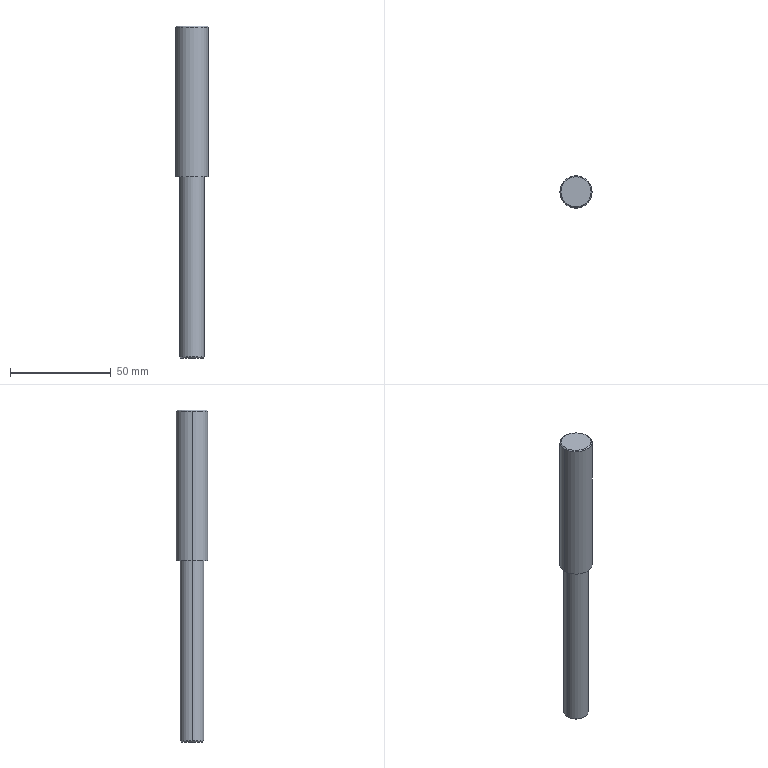Part | STEP file | X77b-01008 | 1 solid | 18 faces | box 16 x 16 x 165 mm | volume 25170 mm3 | cylinder 8 | cone 6 | plane 4 | commonest cylinder face diameters 2.5 x2 3 x2 12 x2 16 x2
STEP:
#1=CARTESIAN_POINT('',(22.255,-49.502,-165.));
#2=VERTEX_POINT('',#1);
#3=CARTESIAN_POINT('',(33.255,-49.502,-165.));
#4=VERTEX_POINT('',#3);
#5=CARTESIAN_POINT('',(27.755,-49.502,-165.));
#6=DIRECTION('',(0.,0.,-1.));
#7=DIRECTION('',(-1.,0.,0.));
#8=AXIS2_PLACEMENT_3D('',#5,#6,#7);
#9=CIRCLE('',#8,5.5);
#10=EDGE_CURVE('',#2,#4,#9,.T.);
#11=ORIENTED_EDGE('',*,*,#10,.F.);
#12=CARTESIAN_POINT('',(21.755,-49.502,-164.5));
#13=VERTEX_POINT('',#12);
#14=CARTESIAN_POINT('',(22.255,-49.502,-165.));
#15=DIRECTION('',(-0.7071,0.,0.7071));
#16=VECTOR('',#15,1000.);
#17=LINE('',#14,#16);
#18=EDGE_CURVE('',#2,#13,#17,.T.);
#19=ORIENTED_EDGE('',*,*,#18,.T.);
#20=CARTESIAN_POINT('',(33.755,-49.502,-164.5));
#21=VERTEX_POINT('',#20);
#22=CARTESIAN_POINT('',(27.755,-49.502,-164.5));
#23=DIRECTION('',(0.,0.,1.));
#24=DIRECTION('',(-1.,0.,0.));
#25=AXIS2_PLACEMENT_3D('',#22,#23,#24);
#26=CIRCLE('',#25,6.);
#27=EDGE_CURVE('',#21,#13,#26,.T.);
#28=ORIENTED_EDGE('',*,*,#27,.F.);
#29=CARTESIAN_POINT('',(33.255,-49.502,-165.));
#30=DIRECTION('',(0.7071,0.,0.7071));
#31=VECTOR('',#30,1000.);
#32=LINE('',#29,#31);
#33=EDGE_CURVE('',#4,#21,#32,.T.);
#34=ORIENTED_EDGE('',*,*,#33,.F.);
#35=EDGE_LOOP('',(#11,#19,#28,#34));
#36=FACE_OUTER_BOUND('',#35,.T.);
#37=CARTESIAN_POINT('',(27.755,-49.502,-165.));
#38=DIRECTION('',(0.,0.,1.));
#39=DIRECTION('',(1.,0.,0.));
#40=AXIS2_PLACEMENT_3D('',#37,#38,#39);
#41=CONICAL_SURFACE('',#40,5.5,0.7854);
#42=ADVANCED_FACE('',(#36),#41,.T.);
#43=CARTESIAN_POINT('',(35.255,-49.502,0.));
#44=VERTEX_POINT('',#43);
#45=CARTESIAN_POINT('',(20.255,-49.502,0.));
#46=VERTEX_POINT('',#45);
#47=CARTESIAN_POINT('',(27.755,-49.502,0.));
#48=DIRECTION('',(0.,0.,1.));
#49=DIRECTION('',(1.,0.,0.));
#50=AXIS2_PLACEMENT_3D('',#47,#48,#49);
#51=CIRCLE('',#50,7.5);
#52=EDGE_CURVE('',#44,#46,#51,.T.);
#53=ORIENTED_EDGE('',*,*,#52,.F.);
#54=CARTESIAN_POINT('',(35.755,-49.502,-0.5));
#55=VERTEX_POINT('',#54);
#56=CARTESIAN_POINT('',(35.255,-49.502,0.));
#57=DIRECTION('',(0.7071,0.,-0.7071));
#58=VECTOR('',#57,1000.);
#59=LINE('',#56,#58);
#60=EDGE_CURVE('',#44,#55,#59,.T.);
#61=ORIENTED_EDGE('',*,*,#60,.T.);
#62=CARTESIAN_POINT('',(19.755,-49.502,-0.5));
#63=VERTEX_POINT('',#62);
#64=CARTESIAN_POINT('',(27.755,-49.502,-0.5));
#65=DIRECTION('',(0.,0.,-1.));
#66=DIRECTION('',(1.,0.,0.));
#67=AXIS2_PLACEMENT_3D('',#64,#65,#66);
#68=CIRCLE('',#67,8.);
#69=EDGE_CURVE('',#63,#55,#68,.T.);
#70=ORIENTED_EDGE('',*,*,#69,.F.);
#71=CARTESIAN_POINT('',(20.255,-49.502,0.));
#72=DIRECTION('',(-0.7071,0.,-0.7071));
#73=VECTOR('',#72,1000.);
#74=LINE('',#71,#73);
#75=EDGE_CURVE('',#46,#63,#74,.T.);
#76=ORIENTED_EDGE('',*,*,#75,.F.);
#77=EDGE_LOOP('',(#53,#61,#70,#76));
#78=FACE_OUTER_BOUND('',#77,.T.);
#79=CARTESIAN_POINT('',(27.755,-49.502,0.));
#80=DIRECTION('',(0.,0.,-1.));
#81=DIRECTION('',(-1.,0.,0.));
#82=AXIS2_PLACEMENT_3D('',#79,#80,#81);
#83=CONICAL_SURFACE('',#82,7.5,0.7854);
#84=ADVANCED_FACE('',(#78),#83,.T.);
#85=CARTESIAN_POINT('',(29.255,-49.502,-157.));
#86=VERTEX_POINT('',#85);
#87=CARTESIAN_POINT('',(26.255,-49.502,-157.));
#88=VERTEX_POINT('',#87);
#89=CARTESIAN_POINT('',(27.755,-49.502,-157.));
#90=DIRECTION('',(0.,0.,-1.));
#91=DIRECTION('',(-1.,0.,0.));
#92=AXIS2_PLACEMENT_3D('',#89,#90,#91);
#93=CIRCLE('',#92,1.5);
#94=EDGE_CURVE('',#86,#88,#93,.T.);
#95=ORIENTED_EDGE('',*,*,#94,.F.);
#96=CARTESIAN_POINT('',(29.255,-49.502,-165.));
#97=VERTEX_POINT('',#96);
#98=CARTESIAN_POINT('',(29.255,-49.502,-165.));
#99=DIRECTION('',(0.,0.,-1.));
#100=VECTOR('',#99,1000.);
#101=LINE('',#98,#100);
#102=EDGE_CURVE('',#86,#97,#101,.T.);
#103=ORIENTED_EDGE('',*,*,#102,.T.);
#104=CARTESIAN_POINT('',(26.255,-49.502,-165.));
#105=VERTEX_POINT('',#104);
#106=CARTESIAN_POINT('',(27.755,-49.502,-165.));
#107=DIRECTION('',(0.,0.,-1.));
#108=DIRECTION('',(-1.,0.,0.));
#109=AXIS2_PLACEMENT_3D('',#106,#107,#108);
#110=CIRCLE('',#109,1.5);
#111=EDGE_CURVE('',#97,#105,#110,.T.);
#112=ORIENTED_EDGE('',*,*,#111,.T.);
#113=CARTESIAN_POINT('',(26.255,-49.502,-165.));
#114=DIRECTION('',(0.,0.,-1.));
#115=VECTOR('',#114,1000.);
#116=LINE('',#113,#115);
#117=EDGE_CURVE('',#88,#105,#116,.T.);
#118=ORIENTED_EDGE('',*,*,#117,.F.);
#119=EDGE_LOOP('',(#95,#103,#112,#118));
#120=FACE_OUTER_BOUND('',#119,.T.);
#121=CARTESIAN_POINT('',(27.755,-49.502,-165.));
#122=DIRECTION('',(0.,0.,-1.));
#123=DIRECTION('',(-1.,0.,0.));
#124=AXIS2_PLACEMENT_3D('',#121,#122,#123);
#125=CYLINDRICAL_SURFACE('',#124,1.5);
#126=ADVANCED_FACE('',(#120),#125,.F.);
#127=CARTESIAN_POINT('',(29.005,-49.502,-153.));
#128=VERTEX_POINT('',#127);
#129=CARTESIAN_POINT('',(26.505,-49.502,-153.));
#130=VERTEX_POINT('',#129);
#131=CARTESIAN_POINT('',(27.755,-49.502,-153.));
#132=DIRECTION('',(0.,0.,-1.));
#133=DIRECTION('',(-1.,0.,0.));
#134=AXIS2_PLACEMENT_3D('',#131,#132,#133);
#135=CIRCLE('',#134,1.25);
#136=EDGE_CURVE('',#128,#130,#135,.T.);
#137=ORIENTED_EDGE('',*,*,#136,.F.);
#138=CARTESIAN_POINT('',(29.005,-49.502,-157.));
#139=VERTEX_POINT('',#138);
#140=CARTESIAN_POINT('',(29.005,-49.502,-165.));
#141=DIRECTION('',(0.,0.,-1.));
#142=VECTOR('',#141,1000.);
#143=LINE('',#140,#142);
#144=EDGE_CURVE('',#128,#139,#143,.T.);
#145=ORIENTED_EDGE('',*,*,#144,.T.);
#146=CARTESIAN_POINT('',(26.505,-49.502,-157.));
#147=VERTEX_POINT('',#146);
#148=CARTESIAN_POINT('',(27.755,-49.502,-157.));
#149=DIRECTION('',(0.,0.,-1.));
#150=DIRECTION('',(-1.,0.,0.));
#151=AXIS2_PLACEMENT_3D('',#148,#149,#150);
#152=CIRCLE('',#151,1.25);
#153=EDGE_CURVE('',#139,#147,#152,.T.);
#154=ORIENTED_EDGE('',*,*,#153,.T.);
#155=CARTESIAN_POINT('',(26.505,-49.502,-165.));
#156=DIRECTION('',(0.,0.,-1.));
#157=VECTOR('',#156,1000.);
#158=LINE('',#155,#157);
#159=EDGE_CURVE('',#130,#147,#158,.T.);
#160=ORIENTED_EDGE('',*,*,#159,.F.);
#161=EDGE_LOOP('',(#137,#145,#154,#160));
#162=FACE_OUTER_BOUND('',#161,.T.);
#163=CARTESIAN_POINT('',(27.755,-49.502,-165.));
#164=DIRECTION('',(0.,0.,-1.));
#165=DIRECTION('',(-1.,0.,0.));
#166=AXIS2_PLACEMENT_3D('',#163,#164,#165);
#167=CYLINDRICAL_SURFACE('',#166,1.25);
#168=ADVANCED_FACE('',(#162),#167,.F.);
#169=CARTESIAN_POINT('',(27.755,-49.502,-152.249));
#170=VERTEX_POINT('',#169);
#171=CARTESIAN_POINT('',(26.505,-49.502,-153.));
#172=DIRECTION('',(-0.8572,0.,-0.515));
#173=VECTOR('',#172,1000.);
#174=LINE('',#171,#173);
#175=EDGE_CURVE('',#170,#130,#174,.T.);
#176=ORIENTED_EDGE('',*,*,#175,.F.);
#177=CARTESIAN_POINT('',(29.005,-49.502,-153.));
#178=DIRECTION('',(0.8572,0.,-0.515));
#179=VECTOR('',#178,1000.);
#180=LINE('',#177,#179);
#181=EDGE_CURVE('',#170,#128,#180,.T.);
#182=ORIENTED_EDGE('',*,*,#181,.T.);
#183=ORIENTED_EDGE('',*,*,#136,.T.);
#184=EDGE_LOOP('',(#176,#182,#183));
#185=FACE_OUTER_BOUND('',#184,.T.);
#186=CARTESIAN_POINT('',(27.755,-49.502,-153.));
#187=DIRECTION('',(0.,0.,-1.));
#188=DIRECTION('',(-1.,0.,0.));
#189=AXIS2_PLACEMENT_3D('',#186,#187,#188);
#190=CONICAL_SURFACE('',#189,1.25,1.03);
#191=ADVANCED_FACE('',(#185),#190,.F.);
#192=ORIENTED_EDGE('',*,*,#27,.T.);
#193=CARTESIAN_POINT('',(21.755,-49.502,-75.));
#194=VERTEX_POINT('',#193);
#195=CARTESIAN_POINT('',(21.755,-49.502,-165.));
#196=DIRECTION('',(0.,0.,1.));
#197=VECTOR('',#196,1000.);
#198=LINE('',#195,#197);
#199=EDGE_CURVE('',#13,#194,#198,.T.);
#200=ORIENTED_EDGE('',*,*,#199,.T.);
#201=CARTESIAN_POINT('',(33.755,-49.502,-75.));
#202=VERTEX_POINT('',#201);
#203=CARTESIAN_POINT('',(27.755,-49.502,-75.));
#204=DIRECTION('',(0.,0.,-1.));
#205=DIRECTION('',(1.,0.,0.));
#206=AXIS2_PLACEMENT_3D('',#203,#204,#205);
#207=CIRCLE('',#206,6.);
#208=EDGE_CURVE('',#194,#202,#207,.T.);
#209=ORIENTED_EDGE('',*,*,#208,.T.);
#210=CARTESIAN_POINT('',(33.755,-49.502,-165.));
#211=DIRECTION('',(0.,0.,1.));
#212=VECTOR('',#211,1000.);
#213=LINE('',#210,#212);
#214=EDGE_CURVE('',#21,#202,#213,.T.);
#215=ORIENTED_EDGE('',*,*,#214,.F.);
#216=EDGE_LOOP('',(#192,#200,#209,#215));
#217=FACE_OUTER_BOUND('',#216,.T.);
#218=CARTESIAN_POINT('',(27.755,-49.502,-165.));
#219=DIRECTION('',(0.,0.,1.));
#220=DIRECTION('',(1.,0.,0.));
#221=AXIS2_PLACEMENT_3D('',#218,#219,#220);
#222=CYLINDRICAL_SURFACE('',#221,6.);
#223=ADVANCED_FACE('',(#217),#222,.T.);
#224=CARTESIAN_POINT('',(35.755,-49.502,-75.));
#225=VERTEX_POINT('',#224);
#226=CARTESIAN_POINT('',(19.755,-49.502,-75.));
#227=VERTEX_POINT('',#226);
#228=CARTESIAN_POINT('',(27.755,-49.502,-75.));
#229=DIRECTION('',(0.,0.,1.));
#230=DIRECTION('',(1.,0.,0.));
#231=AXIS2_PLACEMENT_3D('',#228,#229,#230);
#232=CIRCLE('',#231,8.);
#233=EDGE_CURVE('',#225,#227,#232,.T.);
#234=ORIENTED_EDGE('',*,*,#233,.T.);
#235=CARTESIAN_POINT('',(19.755,-49.502,-75.));
#236=DIRECTION('',(0.,0.,1.));
#237=VECTOR('',#236,1000.);
#238=LINE('',#235,#237);
#239=EDGE_CURVE('',#227,#63,#238,.T.);
#240=ORIENTED_EDGE('',*,*,#239,.T.);
#241=ORIENTED_EDGE('',*,*,#69,.T.);
#242=CARTESIAN_POINT('',(35.755,-49.502,-75.));
#243=DIRECTION('',(0.,0.,1.));
#244=VECTOR('',#243,1000.);
#245=LINE('',#242,#244);
#246=EDGE_CURVE('',#225,#55,#245,.T.);
#247=ORIENTED_EDGE('',*,*,#246,.F.);
#248=EDGE_LOOP('',(#234,#240,#241,#247));
#249=FACE_OUTER_BOUND('',#248,.T.);
#250=CARTESIAN_POINT('',(27.755,-49.502,-75.));
#251=DIRECTION('',(0.,0.,1.));
#252=DIRECTION('',(1.,0.,0.));
#253=AXIS2_PLACEMENT_3D('',#250,#251,#252);
#254=CYLINDRICAL_SURFACE('',#253,8.);
#255=ADVANCED_FACE('',(#249),#254,.T.);
#256=ORIENTED_EDGE('',*,*,#233,.F.);
#257=CARTESIAN_POINT('',(27.755,-49.502,-75.));
#258=DIRECTION('',(0.,0.,1.));
#259=DIRECTION('',(1.,0.,0.));
#260=AXIS2_PLACEMENT_3D('',#257,#258,#259);
#261=CIRCLE('',#260,8.);
#262=EDGE_CURVE('',#227,#225,#261,.T.);
#263=ORIENTED_EDGE('',*,*,#262,.F.);
#264=EDGE_LOOP('',(#256,#263));
#265=FACE_OUTER_BOUND('',#264,.T.);
#266=CARTESIAN_POINT('',(27.755,-49.502,-75.));
#267=DIRECTION('',(0.,0.,-1.));
#268=DIRECTION('',(1.,0.,0.));
#269=AXIS2_PLACEMENT_3D('',#266,#267,#268);
#270=CIRCLE('',#269,6.);
#271=EDGE_CURVE('',#202,#194,#270,.T.);
#272=ORIENTED_EDGE('',*,*,#271,.F.);
#273=ORIENTED_EDGE('',*,*,#208,.F.);
#274=EDGE_LOOP('',(#272,#273));
#275=FACE_BOUND('',#274,.T.);
#276=CARTESIAN_POINT('',(27.755,-49.502,-75.));
#277=DIRECTION('',(0.,0.,1.));
#278=DIRECTION('',(1.,0.,0.));
#279=AXIS2_PLACEMENT_3D('',#276,#277,#278);
#280=PLANE('',#279);
#281=ADVANCED_FACE('',(#265,#275),#280,.F.);
#282=ORIENTED_EDGE('',*,*,#239,.F.);
#283=ORIENTED_EDGE('',*,*,#262,.T.);
#284=ORIENTED_EDGE('',*,*,#246,.T.);
#285=CARTESIAN_POINT('',(27.755,-49.502,-0.5));
#286=DIRECTION('',(0.,0.,-1.));
#287=DIRECTION('',(1.,0.,0.));
#288=AXIS2_PLACEMENT_3D('',#285,#286,#287);
#289=CIRCLE('',#288,8.);
#290=EDGE_CURVE('',#55,#63,#289,.T.);
#291=ORIENTED_EDGE('',*,*,#290,.T.);
#292=EDGE_LOOP('',(#282,#283,#284,#291));
#293=FACE_OUTER_BOUND('',#292,.T.);
#294=CARTESIAN_POINT('',(27.755,-49.502,-75.));
#295=DIRECTION('',(0.,0.,1.));
#296=DIRECTION('',(1.,0.,0.));
#297=AXIS2_PLACEMENT_3D('',#294,#295,#296);
#298=CYLINDRICAL_SURFACE('',#297,8.);
#299=ADVANCED_FACE('',(#293),#298,.T.);
#300=CARTESIAN_POINT('',(27.755,-49.502,0.));
#301=DIRECTION('',(0.,0.,1.));
#302=DIRECTION('',(1.,0.,0.));
#303=AXIS2_PLACEMENT_3D('',#300,#301,#302);
#304=CIRCLE('',#303,7.5);
#305=EDGE_CURVE('',#46,#44,#304,.T.);
#306=ORIENTED_EDGE('',*,*,#305,.T.);
#307=ORIENTED_EDGE('',*,*,#52,.T.);
#308=EDGE_LOOP('',(#306,#307));
#309=FACE_OUTER_BOUND('',#308,.T.);
#310=CARTESIAN_POINT('',(27.755,-49.502,0.));
#311=DIRECTION('',(0.,0.,1.));
#312=DIRECTION('',(1.,0.,0.));
#313=AXIS2_PLACEMENT_3D('',#310,#311,#312);
#314=PLANE('',#313);
#315=ADVANCED_FACE('',(#309),#314,.T.);
#316=ORIENTED_EDGE('',*,*,#199,.F.);
#317=CARTESIAN_POINT('',(27.755,-49.502,-164.5));
#318=DIRECTION('',(0.,0.,1.));
#319=DIRECTION('',(-1.,0.,0.));
#320=AXIS2_PLACEMENT_3D('',#317,#318,#319);
#321=CIRCLE('',#320,6.);
#322=EDGE_CURVE('',#13,#21,#321,.T.);
#323=ORIENTED_EDGE('',*,*,#322,.T.);
#324=ORIENTED_EDGE('',*,*,#214,.T.);
#325=ORIENTED_EDGE('',*,*,#271,.T.);
#326=EDGE_LOOP('',(#316,#323,#324,#325));
#327=FACE_OUTER_BOUND('',#326,.T.);
#328=CARTESIAN_POINT('',(27.755,-49.502,-165.));
#329=DIRECTION('',(0.,0.,1.));
#330=DIRECTION('',(1.,0.,0.));
#331=AXIS2_PLACEMENT_3D('',#328,#329,#330);
#332=CYLINDRICAL_SURFACE('',#331,6.);
#333=ADVANCED_FACE('',(#327),#332,.T.);
#334=CARTESIAN_POINT('',(27.755,-49.502,-165.));
#335=DIRECTION('',(0.,0.,-1.));
#336=DIRECTION('',(-1.,0.,0.));
#337=AXIS2_PLACEMENT_3D('',#334,#335,#336);
#338=CIRCLE('',#337,5.5);
#339=EDGE_CURVE('',#4,#2,#338,.T.);
#340=ORIENTED_EDGE('',*,*,#339,.T.);
#341=ORIENTED_EDGE('',*,*,#10,.T.);
#342=EDGE_LOOP('',(#340,#341));
#343=FACE_OUTER_BOUND('',#342,.T.);
#344=CARTESIAN_POINT('',(27.755,-49.502,-165.));
#345=DIRECTION('',(0.,0.,-1.));
#346=DIRECTION('',(-1.,0.,0.));
#347=AXIS2_PLACEMENT_3D('',#344,#345,#346);
#348=CIRCLE('',#347,1.5);
#349=EDGE_CURVE('',#105,#97,#348,.T.);
#350=ORIENTED_EDGE('',*,*,#349,.F.);
#351=ORIENTED_EDGE('',*,*,#111,.F.);
#352=EDGE_LOOP('',(#350,#351));
#353=FACE_BOUND('',#352,.T.);
#354=CARTESIAN_POINT('',(27.755,-49.502,-165.));
#355=DIRECTION('',(0.,0.,-1.));
#356=DIRECTION('',(-1.,0.,0.));
#357=AXIS2_PLACEMENT_3D('',#354,#355,#356);
#358=PLANE('',#357);
#359=ADVANCED_FACE('',(#343,#353),#358,.T.);
#360=ORIENTED_EDGE('',*,*,#181,.F.);
#361=ORIENTED_EDGE('',*,*,#175,.T.);
#362=CARTESIAN_POINT('',(27.755,-49.502,-153.));
#363=DIRECTION('',(0.,0.,-1.));
#364=DIRECTION('',(-1.,0.,0.));
#365=AXIS2_PLACEMENT_3D('',#362,#363,#364);
#366=CIRCLE('',#365,1.25);
#367=EDGE_CURVE('',#130,#128,#366,.T.);
#368=ORIENTED_EDGE('',*,*,#367,.T.);
#369=EDGE_LOOP('',(#360,#361,#368));
#370=FACE_OUTER_BOUND('',#369,.T.);
#371=CARTESIAN_POINT('',(27.755,-49.502,-153.));
#372=DIRECTION('',(0.,0.,-1.));
#373=DIRECTION('',(-1.,0.,0.));
#374=AXIS2_PLACEMENT_3D('',#371,#372,#373);
#375=CONICAL_SURFACE('',#374,1.25,1.03);
#376=ADVANCED_FACE('',(#370),#375,.F.);
#377=ORIENTED_EDGE('',*,*,#144,.F.);
#378=ORIENTED_EDGE('',*,*,#367,.F.);
#379=ORIENTED_EDGE('',*,*,#159,.T.);
#380=CARTESIAN_POINT('',(27.755,-49.502,-157.));
#381=DIRECTION('',(0.,0.,-1.));
#382=DIRECTION('',(-1.,0.,0.));
#383=AXIS2_PLACEMENT_3D('',#380,#381,#382);
#384=CIRCLE('',#383,1.25);
#385=EDGE_CURVE('',#147,#139,#384,.T.);
#386=ORIENTED_EDGE('',*,*,#385,.T.);
#387=EDGE_LOOP('',(#377,#378,#379,#386));
#388=FACE_OUTER_BOUND('',#387,.T.);
#389=CARTESIAN_POINT('',(27.755,-49.502,-165.));
#390=DIRECTION('',(0.,0.,-1.));
#391=DIRECTION('',(-1.,0.,0.));
#392=AXIS2_PLACEMENT_3D('',#389,#390,#391);
#393=CYLINDRICAL_SURFACE('',#392,1.25);
#394=ADVANCED_FACE('',(#388),#393,.F.);
#395=ORIENTED_EDGE('',*,*,#385,.F.);
#396=ORIENTED_EDGE('',*,*,#153,.F.);
#397=EDGE_LOOP('',(#395,#396));
#398=FACE_BOUND('',#397,.T.);
#399=CARTESIAN_POINT('',(27.755,-49.502,-157.));
#400=DIRECTION('',(0.,0.,-1.));
#401=DIRECTION('',(-1.,0.,0.));
#402=AXIS2_PLACEMENT_3D('',#399,#400,#401);
#403=CIRCLE('',#402,1.5);
#404=EDGE_CURVE('',#88,#86,#403,.T.);
#405=ORIENTED_EDGE('',*,*,#404,.T.);
#406=ORIENTED_EDGE('',*,*,#94,.T.);
#407=EDGE_LOOP('',(#405,#406));
#408=FACE_OUTER_BOUND('',#407,.T.);
#409=CARTESIAN_POINT('',(29.005,-49.502,-157.));
#410=DIRECTION('',(0.,0.,1.));
#411=DIRECTION('',(1.,0.,0.));
#412=AXIS2_PLACEMENT_3D('',#409,#410,#411);
#413=PLANE('',#412);
#414=ADVANCED_FACE('',(#398,#408),#413,.F.);
#415=ORIENTED_EDGE('',*,*,#102,.F.);
#416=ORIENTED_EDGE('',*,*,#404,.F.);
#417=ORIENTED_EDGE('',*,*,#117,.T.);
#418=ORIENTED_EDGE('',*,*,#349,.T.);
#419=EDGE_LOOP('',(#415,#416,#417,#418));
#420=FACE_OUTER_BOUND('',#419,.T.);
#421=CARTESIAN_POINT('',(27.755,-49.502,-165.));
#422=DIRECTION('',(0.,0.,-1.));
#423=DIRECTION('',(-1.,0.,0.));
#424=AXIS2_PLACEMENT_3D('',#421,#422,#423);
#425=CYLINDRICAL_SURFACE('',#424,1.5);
#426=ADVANCED_FACE('',(#420),#425,.F.);
#427=ORIENTED_EDGE('',*,*,#60,.F.);
#428=ORIENTED_EDGE('',*,*,#305,.F.);
#429=ORIENTED_EDGE('',*,*,#75,.T.);
#430=ORIENTED_EDGE('',*,*,#290,.F.);
#431=EDGE_LOOP('',(#427,#428,#429,#430));
#432=FACE_OUTER_BOUND('',#431,.T.);
#433=CARTESIAN_POINT('',(27.755,-49.502,0.));
#434=DIRECTION('',(0.,0.,-1.));
#435=DIRECTION('',(-1.,0.,0.));
#436=AXIS2_PLACEMENT_3D('',#433,#434,#435);
#437=CONICAL_SURFACE('',#436,7.5,0.7854);
#438=ADVANCED_FACE('',(#432),#437,.T.);
#439=ORIENTED_EDGE('',*,*,#18,.F.);
#440=ORIENTED_EDGE('',*,*,#339,.F.);
#441=ORIENTED_EDGE('',*,*,#33,.T.);
#442=ORIENTED_EDGE('',*,*,#322,.F.);
#443=EDGE_LOOP('',(#439,#440,#441,#442));
#444=FACE_OUTER_BOUND('',#443,.T.);
#445=CARTESIAN_POINT('',(27.755,-49.502,-165.));
#446=DIRECTION('',(0.,0.,1.));
#447=DIRECTION('',(1.,0.,0.));
#448=AXIS2_PLACEMENT_3D('',#445,#446,#447);
#449=CONICAL_SURFACE('',#448,5.5,0.7854);
#450=ADVANCED_FACE('',(#444),#449,.T.);
#451=CLOSED_SHELL('',(#42,#84,#126,#168,#191,#223,#255,#281,#299,#315,#333,#359,#376,#394,#414,#426,#438,#450));
#452=MANIFOLD_SOLID_BREP('',#451);
#453=CARTESIAN_POINT('',(0.,0.,0.));
#454=DIRECTION('',(0.,0.,1.));
#455=DIRECTION('',(1.,0.,0.));
#456=AXIS2_PLACEMENT_3D('',#453,#454,#455);
#457=(LENGTH_UNIT()NAMED_UNIT(*)SI_UNIT(.MILLI.,.METRE.));
#458=UNCERTAINTY_MEASURE_WITH_UNIT(LENGTH_MEASURE(0.00001),#457,'','');
#459=(NAMED_UNIT(*)PLANE_ANGLE_UNIT()SI_UNIT($,.RADIAN.));
#460=(NAMED_UNIT(*)SI_UNIT($,.STERADIAN.)SOLID_ANGLE_UNIT());
#461=(GEOMETRIC_REPRESENTATION_CONTEXT(3)GLOBAL_UNCERTAINTY_ASSIGNED_CONTEXT((#458))GLOBAL_UNIT_ASSIGNED_CONTEXT((#457,#459,#460))REPRESENTATION_CONTEXT('',''));
#462=ADVANCED_BREP_SHAPE_REPRESENTATION('',(#452,#456),#461);